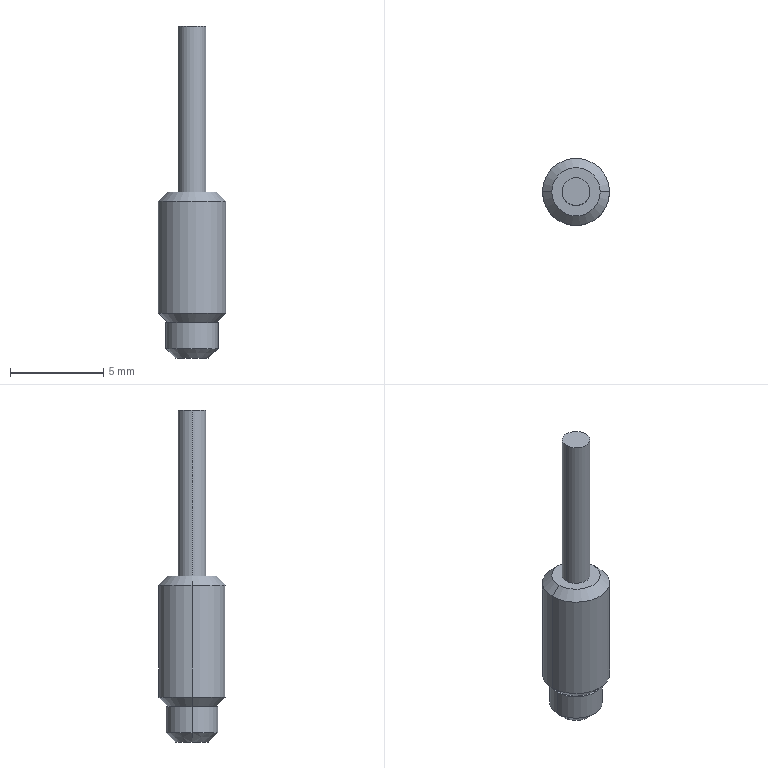Part | SolidWorks | features Chamfer 3, Boss 2, Extrusion 1 | 1 solid | 16 faces | box 3.6 x 3.6 x 17.8 mm | volume 95.144 mm3 | cone 6 | cylinder 6 | plane 4 | commonest cylinder face diameters 1.5 x2 2.8 x2 3.6 x2
STEP:
#1=CARTESIAN_POINT('',(-0.9,0.,-1.9));
#2=VERTEX_POINT('',#1);
#3=CARTESIAN_POINT('',(0.9,0.,-1.9));
#4=VERTEX_POINT('',#3);
#5=CARTESIAN_POINT('',(0.,0.,-1.9));
#6=DIRECTION('',(0.,0.,-1.));
#7=DIRECTION('',(-1.,0.,0.));
#8=AXIS2_PLACEMENT_3D('',#5,#6,#7);
#9=CIRCLE('',#8,0.9);
#10=EDGE_CURVE('',#2,#4,#9,.T.);
#11=ORIENTED_EDGE('',*,*,#10,.F.);
#12=CARTESIAN_POINT('',(-1.4,0.,-1.4));
#13=VERTEX_POINT('',#12);
#14=CARTESIAN_POINT('',(-0.9,0.,-1.9));
#15=DIRECTION('',(-0.7071,0.,0.7071));
#16=VECTOR('',#15,1000.);
#17=LINE('',#14,#16);
#18=EDGE_CURVE('',#2,#13,#17,.T.);
#19=ORIENTED_EDGE('',*,*,#18,.T.);
#20=CARTESIAN_POINT('',(1.4,0.,-1.4));
#21=VERTEX_POINT('',#20);
#22=CARTESIAN_POINT('',(0.,0.,-1.4));
#23=DIRECTION('',(0.,0.,1.));
#24=DIRECTION('',(-1.,0.,0.));
#25=AXIS2_PLACEMENT_3D('',#22,#23,#24);
#26=CIRCLE('',#25,1.4);
#27=EDGE_CURVE('',#21,#13,#26,.T.);
#28=ORIENTED_EDGE('',*,*,#27,.F.);
#29=CARTESIAN_POINT('',(0.9,0.,-1.9));
#30=DIRECTION('',(0.7071,0.,0.7071));
#31=VECTOR('',#30,1000.);
#32=LINE('',#29,#31);
#33=EDGE_CURVE('',#4,#21,#32,.T.);
#34=ORIENTED_EDGE('',*,*,#33,.F.);
#35=EDGE_LOOP('',(#11,#19,#28,#34));
#36=FACE_OUTER_BOUND('',#35,.T.);
#37=CARTESIAN_POINT('',(0.,0.,-1.9));
#38=DIRECTION('',(0.,0.,1.));
#39=DIRECTION('',(1.,0.,0.));
#40=AXIS2_PLACEMENT_3D('',#37,#38,#39);
#41=CONICAL_SURFACE('',#40,0.9,0.7854);
#42=ADVANCED_FACE('',(#36),#41,.T.);
#43=ORIENTED_EDGE('',*,*,#27,.T.);
#44=CARTESIAN_POINT('',(-1.4,0.,0.));
#45=VERTEX_POINT('',#44);
#46=CARTESIAN_POINT('',(-1.4,0.,-1.9));
#47=DIRECTION('',(0.,0.,1.));
#48=VECTOR('',#47,1000.);
#49=LINE('',#46,#48);
#50=EDGE_CURVE('',#13,#45,#49,.T.);
#51=ORIENTED_EDGE('',*,*,#50,.T.);
#52=CARTESIAN_POINT('',(1.4,0.,0.));
#53=VERTEX_POINT('',#52);
#54=CARTESIAN_POINT('',(0.,0.,0.));
#55=DIRECTION('',(0.,0.,-1.));
#56=DIRECTION('',(-1.,0.,0.));
#57=AXIS2_PLACEMENT_3D('',#54,#55,#56);
#58=CIRCLE('',#57,1.4);
#59=EDGE_CURVE('',#45,#53,#58,.T.);
#60=ORIENTED_EDGE('',*,*,#59,.T.);
#61=CARTESIAN_POINT('',(1.4,0.,-1.9));
#62=DIRECTION('',(0.,0.,1.));
#63=VECTOR('',#62,1000.);
#64=LINE('',#61,#63);
#65=EDGE_CURVE('',#21,#53,#64,.T.);
#66=ORIENTED_EDGE('',*,*,#65,.F.);
#67=EDGE_LOOP('',(#43,#51,#60,#66));
#68=FACE_OUTER_BOUND('',#67,.T.);
#69=CARTESIAN_POINT('',(0.,0.,-1.9));
#70=DIRECTION('',(0.,0.,1.));
#71=DIRECTION('',(1.,0.,0.));
#72=AXIS2_PLACEMENT_3D('',#69,#70,#71);
#73=CYLINDRICAL_SURFACE('',#72,1.4);
#74=ADVANCED_FACE('',(#68),#73,.T.);
#75=CARTESIAN_POINT('',(1.3,0.,7.));
#76=VERTEX_POINT('',#75);
#77=CARTESIAN_POINT('',(-1.3,0.,7.));
#78=VERTEX_POINT('',#77);
#79=CARTESIAN_POINT('',(0.,0.,7.));
#80=DIRECTION('',(0.,0.,1.));
#81=DIRECTION('',(1.,0.,0.));
#82=AXIS2_PLACEMENT_3D('',#79,#80,#81);
#83=CIRCLE('',#82,1.3);
#84=EDGE_CURVE('',#76,#78,#83,.T.);
#85=ORIENTED_EDGE('',*,*,#84,.F.);
#86=CARTESIAN_POINT('',(1.8,0.,6.5));
#87=VERTEX_POINT('',#86);
#88=CARTESIAN_POINT('',(1.3,0.,7.));
#89=DIRECTION('',(0.7071,0.,-0.7071));
#90=VECTOR('',#89,1000.);
#91=LINE('',#88,#90);
#92=EDGE_CURVE('',#76,#87,#91,.T.);
#93=ORIENTED_EDGE('',*,*,#92,.T.);
#94=CARTESIAN_POINT('',(-1.8,0.,6.5));
#95=VERTEX_POINT('',#94);
#96=CARTESIAN_POINT('',(0.,0.,6.5));
#97=DIRECTION('',(0.,0.,-1.));
#98=DIRECTION('',(1.,0.,0.));
#99=AXIS2_PLACEMENT_3D('',#96,#97,#98);
#100=CIRCLE('',#99,1.8);
#101=EDGE_CURVE('',#95,#87,#100,.T.);
#102=ORIENTED_EDGE('',*,*,#101,.F.);
#103=CARTESIAN_POINT('',(-1.3,0.,7.));
#104=DIRECTION('',(-0.7071,0.,-0.7071));
#105=VECTOR('',#104,1000.);
#106=LINE('',#103,#105);
#107=EDGE_CURVE('',#78,#95,#106,.T.);
#108=ORIENTED_EDGE('',*,*,#107,.F.);
#109=EDGE_LOOP('',(#85,#93,#102,#108));
#110=FACE_OUTER_BOUND('',#109,.T.);
#111=CARTESIAN_POINT('',(0.,0.,7.));
#112=DIRECTION('',(0.,0.,-1.));
#113=DIRECTION('',(-1.,0.,0.));
#114=AXIS2_PLACEMENT_3D('',#111,#112,#113);
#115=CONICAL_SURFACE('',#114,1.3,0.7854);
#116=ADVANCED_FACE('',(#110),#115,.T.);
#117=CARTESIAN_POINT('',(-1.3,0.,0.));
#118=VERTEX_POINT('',#117);
#119=CARTESIAN_POINT('',(1.3,0.,0.));
#120=VERTEX_POINT('',#119);
#121=CARTESIAN_POINT('',(0.,0.,0.));
#122=DIRECTION('',(0.,0.,-1.));
#123=DIRECTION('',(1.,0.,0.));
#124=AXIS2_PLACEMENT_3D('',#121,#122,#123);
#125=CIRCLE('',#124,1.3);
#126=EDGE_CURVE('',#118,#120,#125,.T.);
#127=ORIENTED_EDGE('',*,*,#126,.F.);
#128=CARTESIAN_POINT('',(-1.8,0.,0.5));
#129=VERTEX_POINT('',#128);
#130=CARTESIAN_POINT('',(-1.8,0.,0.5));
#131=DIRECTION('',(-0.7071,0.,0.7071));
#132=VECTOR('',#131,1000.);
#133=LINE('',#130,#132);
#134=EDGE_CURVE('',#118,#129,#133,.T.);
#135=ORIENTED_EDGE('',*,*,#134,.T.);
#136=CARTESIAN_POINT('',(1.8,0.,0.5));
#137=VERTEX_POINT('',#136);
#138=CARTESIAN_POINT('',(0.,0.,0.5));
#139=DIRECTION('',(0.,0.,1.));
#140=DIRECTION('',(1.,0.,0.));
#141=AXIS2_PLACEMENT_3D('',#138,#139,#140);
#142=CIRCLE('',#141,1.8);
#143=EDGE_CURVE('',#137,#129,#142,.T.);
#144=ORIENTED_EDGE('',*,*,#143,.F.);
#145=CARTESIAN_POINT('',(1.8,0.,0.5));
#146=DIRECTION('',(0.7071,0.,0.7071));
#147=VECTOR('',#146,1000.);
#148=LINE('',#145,#147);
#149=EDGE_CURVE('',#120,#137,#148,.T.);
#150=ORIENTED_EDGE('',*,*,#149,.F.);
#151=EDGE_LOOP('',(#127,#135,#144,#150));
#152=FACE_OUTER_BOUND('',#151,.T.);
#153=CARTESIAN_POINT('',(0.,0.,0.5));
#154=DIRECTION('',(0.,0.,1.));
#155=DIRECTION('',(1.,0.,0.));
#156=AXIS2_PLACEMENT_3D('',#153,#154,#155);
#157=CONICAL_SURFACE('',#156,1.8,0.7854);
#158=ADVANCED_FACE('',(#152),#157,.T.);
#159=CARTESIAN_POINT('',(0.75,0.,15.9));
#160=VERTEX_POINT('',#159);
#161=CARTESIAN_POINT('',(-0.75,0.,15.9));
#162=VERTEX_POINT('',#161);
#163=CARTESIAN_POINT('',(0.,0.,15.9));
#164=DIRECTION('',(0.,0.,1.));
#165=DIRECTION('',(1.,0.,0.));
#166=AXIS2_PLACEMENT_3D('',#163,#164,#165);
#167=CIRCLE('',#166,0.75);
#168=EDGE_CURVE('',#160,#162,#167,.T.);
#169=ORIENTED_EDGE('',*,*,#168,.F.);
#170=CARTESIAN_POINT('',(0.75,0.,7.));
#171=VERTEX_POINT('',#170);
#172=CARTESIAN_POINT('',(0.75,0.,15.9));
#173=DIRECTION('',(0.,0.,-1.));
#174=VECTOR('',#173,1000.);
#175=LINE('',#172,#174);
#176=EDGE_CURVE('',#160,#171,#175,.T.);
#177=ORIENTED_EDGE('',*,*,#176,.T.);
#178=CARTESIAN_POINT('',(-0.75,0.,7.));
#179=VERTEX_POINT('',#178);
#180=CARTESIAN_POINT('',(0.,0.,7.));
#181=DIRECTION('',(0.,0.,1.));
#182=DIRECTION('',(1.,0.,0.));
#183=AXIS2_PLACEMENT_3D('',#180,#181,#182);
#184=CIRCLE('',#183,0.75);
#185=EDGE_CURVE('',#171,#179,#184,.T.);
#186=ORIENTED_EDGE('',*,*,#185,.T.);
#187=CARTESIAN_POINT('',(-0.75,0.,15.9));
#188=DIRECTION('',(0.,0.,-1.));
#189=VECTOR('',#188,1000.);
#190=LINE('',#187,#189);
#191=EDGE_CURVE('',#162,#179,#190,.T.);
#192=ORIENTED_EDGE('',*,*,#191,.F.);
#193=EDGE_LOOP('',(#169,#177,#186,#192));
#194=FACE_OUTER_BOUND('',#193,.T.);
#195=CARTESIAN_POINT('',(0.,0.,15.9));
#196=DIRECTION('',(0.,0.,-1.));
#197=DIRECTION('',(-1.,0.,0.));
#198=AXIS2_PLACEMENT_3D('',#195,#196,#197);
#199=CYLINDRICAL_SURFACE('',#198,0.75);
#200=ADVANCED_FACE('',(#194),#199,.T.);
#201=ORIENTED_EDGE('',*,*,#101,.T.);
#202=CARTESIAN_POINT('',(1.8,0.,7.));
#203=DIRECTION('',(0.,0.,-1.));
#204=VECTOR('',#203,1000.);
#205=LINE('',#202,#204);
#206=EDGE_CURVE('',#87,#137,#205,.T.);
#207=ORIENTED_EDGE('',*,*,#206,.T.);
#208=ORIENTED_EDGE('',*,*,#143,.T.);
#209=CARTESIAN_POINT('',(-1.8,0.,7.));
#210=DIRECTION('',(0.,0.,-1.));
#211=VECTOR('',#210,1000.);
#212=LINE('',#209,#211);
#213=EDGE_CURVE('',#95,#129,#212,.T.);
#214=ORIENTED_EDGE('',*,*,#213,.F.);
#215=EDGE_LOOP('',(#201,#207,#208,#214));
#216=FACE_OUTER_BOUND('',#215,.T.);
#217=CARTESIAN_POINT('',(0.,0.,7.));
#218=DIRECTION('',(0.,0.,-1.));
#219=DIRECTION('',(-1.,0.,0.));
#220=AXIS2_PLACEMENT_3D('',#217,#218,#219);
#221=CYLINDRICAL_SURFACE('',#220,1.8);
#222=ADVANCED_FACE('',(#216),#221,.T.);
#223=CARTESIAN_POINT('',(0.,0.,7.));
#224=DIRECTION('',(0.,0.,1.));
#225=DIRECTION('',(1.,0.,0.));
#226=AXIS2_PLACEMENT_3D('',#223,#224,#225);
#227=CIRCLE('',#226,1.3);
#228=EDGE_CURVE('',#78,#76,#227,.T.);
#229=ORIENTED_EDGE('',*,*,#228,.T.);
#230=ORIENTED_EDGE('',*,*,#84,.T.);
#231=EDGE_LOOP('',(#229,#230));
#232=FACE_OUTER_BOUND('',#231,.T.);
#233=CARTESIAN_POINT('',(0.,0.,7.));
#234=DIRECTION('',(0.,0.,1.));
#235=DIRECTION('',(1.,0.,0.));
#236=AXIS2_PLACEMENT_3D('',#233,#234,#235);
#237=CIRCLE('',#236,0.75);
#238=EDGE_CURVE('',#179,#171,#237,.T.);
#239=ORIENTED_EDGE('',*,*,#238,.F.);
#240=ORIENTED_EDGE('',*,*,#185,.F.);
#241=EDGE_LOOP('',(#239,#240));
#242=FACE_BOUND('',#241,.T.);
#243=CARTESIAN_POINT('',(0.,0.,7.));
#244=DIRECTION('',(0.,0.,1.));
#245=DIRECTION('',(1.,0.,0.));
#246=AXIS2_PLACEMENT_3D('',#243,#244,#245);
#247=PLANE('',#246);
#248=ADVANCED_FACE('',(#232,#242),#247,.T.);
#249=ORIENTED_EDGE('',*,*,#206,.F.);
#250=CARTESIAN_POINT('',(0.,0.,6.5));
#251=DIRECTION('',(0.,0.,-1.));
#252=DIRECTION('',(1.,0.,0.));
#253=AXIS2_PLACEMENT_3D('',#250,#251,#252);
#254=CIRCLE('',#253,1.8);
#255=EDGE_CURVE('',#87,#95,#254,.T.);
#256=ORIENTED_EDGE('',*,*,#255,.T.);
#257=ORIENTED_EDGE('',*,*,#213,.T.);
#258=CARTESIAN_POINT('',(0.,0.,0.5));
#259=DIRECTION('',(0.,0.,1.));
#260=DIRECTION('',(1.,0.,0.));
#261=AXIS2_PLACEMENT_3D('',#258,#259,#260);
#262=CIRCLE('',#261,1.8);
#263=EDGE_CURVE('',#129,#137,#262,.T.);
#264=ORIENTED_EDGE('',*,*,#263,.T.);
#265=EDGE_LOOP('',(#249,#256,#257,#264));
#266=FACE_OUTER_BOUND('',#265,.T.);
#267=CARTESIAN_POINT('',(0.,0.,7.));
#268=DIRECTION('',(0.,0.,-1.));
#269=DIRECTION('',(-1.,0.,0.));
#270=AXIS2_PLACEMENT_3D('',#267,#268,#269);
#271=CYLINDRICAL_SURFACE('',#270,1.8);
#272=ADVANCED_FACE('',(#266),#271,.T.);
#273=ORIENTED_EDGE('',*,*,#176,.F.);
#274=CARTESIAN_POINT('',(0.,0.,15.9));
#275=DIRECTION('',(0.,0.,1.));
#276=DIRECTION('',(1.,0.,0.));
#277=AXIS2_PLACEMENT_3D('',#274,#275,#276);
#278=CIRCLE('',#277,0.75);
#279=EDGE_CURVE('',#162,#160,#278,.T.);
#280=ORIENTED_EDGE('',*,*,#279,.F.);
#281=ORIENTED_EDGE('',*,*,#191,.T.);
#282=ORIENTED_EDGE('',*,*,#238,.T.);
#283=EDGE_LOOP('',(#273,#280,#281,#282));
#284=FACE_OUTER_BOUND('',#283,.T.);
#285=CARTESIAN_POINT('',(0.,0.,15.9));
#286=DIRECTION('',(0.,0.,-1.));
#287=DIRECTION('',(-1.,0.,0.));
#288=AXIS2_PLACEMENT_3D('',#285,#286,#287);
#289=CYLINDRICAL_SURFACE('',#288,0.75);
#290=ADVANCED_FACE('',(#284),#289,.T.);
#291=ORIENTED_EDGE('',*,*,#279,.T.);
#292=ORIENTED_EDGE('',*,*,#168,.T.);
#293=EDGE_LOOP('',(#291,#292));
#294=FACE_OUTER_BOUND('',#293,.T.);
#295=CARTESIAN_POINT('',(0.,0.,15.9));
#296=DIRECTION('',(0.,0.,1.));
#297=DIRECTION('',(1.,0.,0.));
#298=AXIS2_PLACEMENT_3D('',#295,#296,#297);
#299=PLANE('',#298);
#300=ADVANCED_FACE('',(#294),#299,.T.);
#301=ORIENTED_EDGE('',*,*,#134,.F.);
#302=CARTESIAN_POINT('',(0.,0.,0.));
#303=DIRECTION('',(0.,0.,-1.));
#304=DIRECTION('',(1.,0.,0.));
#305=AXIS2_PLACEMENT_3D('',#302,#303,#304);
#306=CIRCLE('',#305,1.3);
#307=EDGE_CURVE('',#120,#118,#306,.T.);
#308=ORIENTED_EDGE('',*,*,#307,.F.);
#309=ORIENTED_EDGE('',*,*,#149,.T.);
#310=ORIENTED_EDGE('',*,*,#263,.F.);
#311=EDGE_LOOP('',(#301,#308,#309,#310));
#312=FACE_OUTER_BOUND('',#311,.T.);
#313=CARTESIAN_POINT('',(0.,0.,0.5));
#314=DIRECTION('',(0.,0.,1.));
#315=DIRECTION('',(1.,0.,0.));
#316=AXIS2_PLACEMENT_3D('',#313,#314,#315);
#317=CONICAL_SURFACE('',#316,1.8,0.7854);
#318=ADVANCED_FACE('',(#312),#317,.T.);
#319=ORIENTED_EDGE('',*,*,#92,.F.);
#320=ORIENTED_EDGE('',*,*,#228,.F.);
#321=ORIENTED_EDGE('',*,*,#107,.T.);
#322=ORIENTED_EDGE('',*,*,#255,.F.);
#323=EDGE_LOOP('',(#319,#320,#321,#322));
#324=FACE_OUTER_BOUND('',#323,.T.);
#325=CARTESIAN_POINT('',(0.,0.,7.));
#326=DIRECTION('',(0.,0.,-1.));
#327=DIRECTION('',(-1.,0.,0.));
#328=AXIS2_PLACEMENT_3D('',#325,#326,#327);
#329=CONICAL_SURFACE('',#328,1.3,0.7854);
#330=ADVANCED_FACE('',(#324),#329,.T.);
#331=ORIENTED_EDGE('',*,*,#50,.F.);
#332=CARTESIAN_POINT('',(0.,0.,-1.4));
#333=DIRECTION('',(0.,0.,1.));
#334=DIRECTION('',(-1.,0.,0.));
#335=AXIS2_PLACEMENT_3D('',#332,#333,#334);
#336=CIRCLE('',#335,1.4);
#337=EDGE_CURVE('',#13,#21,#336,.T.);
#338=ORIENTED_EDGE('',*,*,#337,.T.);
#339=ORIENTED_EDGE('',*,*,#65,.T.);
#340=CARTESIAN_POINT('',(0.,0.,0.));
#341=DIRECTION('',(0.,0.,-1.));
#342=DIRECTION('',(-1.,0.,0.));
#343=AXIS2_PLACEMENT_3D('',#340,#341,#342);
#344=CIRCLE('',#343,1.4);
#345=EDGE_CURVE('',#53,#45,#344,.T.);
#346=ORIENTED_EDGE('',*,*,#345,.T.);
#347=EDGE_LOOP('',(#331,#338,#339,#346));
#348=FACE_OUTER_BOUND('',#347,.T.);
#349=CARTESIAN_POINT('',(0.,0.,-1.9));
#350=DIRECTION('',(0.,0.,1.));
#351=DIRECTION('',(1.,0.,0.));
#352=AXIS2_PLACEMENT_3D('',#349,#350,#351);
#353=CYLINDRICAL_SURFACE('',#352,1.4);
#354=ADVANCED_FACE('',(#348),#353,.T.);
#355=CARTESIAN_POINT('',(0.,0.,-1.9));
#356=DIRECTION('',(0.,0.,-1.));
#357=DIRECTION('',(-1.,0.,0.));
#358=AXIS2_PLACEMENT_3D('',#355,#356,#357);
#359=CIRCLE('',#358,0.9);
#360=EDGE_CURVE('',#4,#2,#359,.T.);
#361=ORIENTED_EDGE('',*,*,#360,.T.);
#362=ORIENTED_EDGE('',*,*,#10,.T.);
#363=EDGE_LOOP('',(#361,#362));
#364=FACE_OUTER_BOUND('',#363,.T.);
#365=CARTESIAN_POINT('',(0.,0.,-1.9));
#366=DIRECTION('',(0.,0.,-1.));
#367=DIRECTION('',(-1.,0.,0.));
#368=AXIS2_PLACEMENT_3D('',#365,#366,#367);
#369=PLANE('',#368);
#370=ADVANCED_FACE('',(#364),#369,.T.);
#371=ORIENTED_EDGE('',*,*,#307,.T.);
#372=ORIENTED_EDGE('',*,*,#126,.T.);
#373=EDGE_LOOP('',(#371,#372));
#374=FACE_BOUND('',#373,.T.);
#375=ORIENTED_EDGE('',*,*,#345,.F.);
#376=ORIENTED_EDGE('',*,*,#59,.F.);
#377=EDGE_LOOP('',(#375,#376));
#378=FACE_OUTER_BOUND('',#377,.T.);
#379=CARTESIAN_POINT('',(0.,0.,0.));
#380=DIRECTION('',(0.,0.,-1.));
#381=DIRECTION('',(-1.,0.,0.));
#382=AXIS2_PLACEMENT_3D('',#379,#380,#381);
#383=PLANE('',#382);
#384=ADVANCED_FACE('',(#374,#378),#383,.F.);
#385=ORIENTED_EDGE('',*,*,#18,.F.);
#386=ORIENTED_EDGE('',*,*,#360,.F.);
#387=ORIENTED_EDGE('',*,*,#33,.T.);
#388=ORIENTED_EDGE('',*,*,#337,.F.);
#389=EDGE_LOOP('',(#385,#386,#387,#388));
#390=FACE_OUTER_BOUND('',#389,.T.);
#391=CARTESIAN_POINT('',(0.,0.,-1.9));
#392=DIRECTION('',(0.,0.,1.));
#393=DIRECTION('',(1.,0.,0.));
#394=AXIS2_PLACEMENT_3D('',#391,#392,#393);
#395=CONICAL_SURFACE('',#394,0.9,0.7854);
#396=ADVANCED_FACE('',(#390),#395,.T.);
#397=CLOSED_SHELL('',(#42,#74,#116,#158,#200,#222,#248,#272,#290,#300,#318,#330,#354,#370,#384,#396));
#398=MANIFOLD_SOLID_BREP('',#397);
#399=CARTESIAN_POINT('',(0.,0.,0.));
#400=DIRECTION('',(0.,0.,1.));
#401=DIRECTION('',(1.,0.,0.));
#402=AXIS2_PLACEMENT_3D('',#399,#400,#401);
#403=(LENGTH_UNIT()NAMED_UNIT(*)SI_UNIT(.MILLI.,.METRE.));
#404=UNCERTAINTY_MEASURE_WITH_UNIT(LENGTH_MEASURE(0.00001),#403,'','');
#405=(NAMED_UNIT(*)PLANE_ANGLE_UNIT()SI_UNIT($,.RADIAN.));
#406=(NAMED_UNIT(*)SI_UNIT($,.STERADIAN.)SOLID_ANGLE_UNIT());
#407=(GEOMETRIC_REPRESENTATION_CONTEXT(3)GLOBAL_UNCERTAINTY_ASSIGNED_CONTEXT((#404))GLOBAL_UNIT_ASSIGNED_CONTEXT((#403,#405,#406))REPRESENTATION_CONTEXT('',''));
#408=ADVANCED_BREP_SHAPE_REPRESENTATION('',(#398,#402),#407);